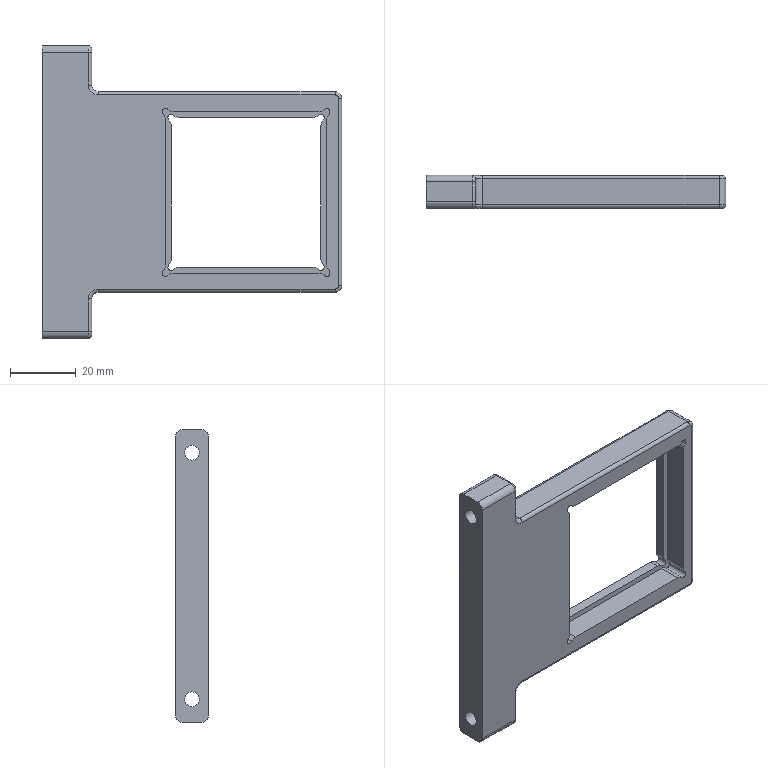CAM job | NX | 3+2 milling | part box 91 x 10 x 89 mm | stock box 96 x 12 x 90 mm
Tools:
number,name,description,diameter,corner_radius,flute_length,length,flutes
4,D4,平底铣刀-粗,4.0,0.0,25.0,75.0,2
9,D10,平底铣刀-粗,10.0,0.0,35.0,75.0,2
17,D2-J,平底铣刀-精,2.0,0.0,50.0,75.0,2
11,D4-J,平底铣刀-精,4.0,0.0,50.0,75.0,2
10,D10-J,平底铣刀-精,10.0,0.0,35.0,75.0,2
19,D4R0.5,圆鼻刀-粗,4.0,0.5,50.0,75.0,2
1,D80R0.8飞刀,圆鼻刀-粗,80.0,0.8,50.0,75.0,2
1,D80R0.8飞刀-J,圆鼻刀-精,80.0,0.8,50.0,75.0,2
2,D6倒角刀,倒角刀,6.0,0.0,3.0,25.0,2
Operations:
program,operation,operation_type,tool,method,geometry_group,spindle_rpm,surface_speed,feed_per_tooth,feed_cut,feed_plunge,cut_length_mm,path_length_mm,cut_time_min,machine_time_min
B,FLOORWALL_FACEMILL_ROUGH_COPY,VolumeBased25DMillingOperation,D80R0.8飞刀,LAYER_ROUGH-DEPTHK-STEPG,W-B,2800.0,703.696,0.5357,3000.0,100.0,1471.688,1680.498,0.4906,0.5114
B,FLOORWALL_FACEMILL_FINISH_COPY,VolumeBased25DMillingOperation,D80R0.8飞刀-J,SIDEFINISH-DEPTHK-STEPG,W-B,4000.0,1005.28,0.125,1000.0,100.0,367.285,463.285,0.3673,0.3769
B,ZLEVEL_FINISH_ZIGZAG_WALL_COPY_COPY_1,ZLevelMilling,D4R0.5,ZLEVEL_WALL-DEPTHK-STEPG,W-B,8000.0,100.531,0.25,4000.0,100.0,1678.657,1818.13,0.4197,0.4336
B,ZLEVEL_FINISH_ZIGZAG_WALL_COPY_COPY_COPY,ZLevelMilling,D4R0.5,ZLEVEL_WALL-DEPTHK-STEPG,W-B,8000.0,100.531,0.25,4000.0,100.0,5427.837,5452.449,1.357,1.359
B,PLANAR_DEBURR_6X45L_COPY,SurfaceContour,D6倒角刀,WALL_CHAMFER-DEPTH0-STEPG,W-B,6500.0,122.519,0.1154,1500.0,100.0,276.36,490.76,0.1842,0.2057
A,TOP_FACE,FaceMilling,D80R0.8飞刀,SIDEFINISH-DEPTHK-STEPG,W-A,4000.0,1005.31,0.125,1000.0,100.0,611.5,647.5,0.6115,0.6151
A,CAVITY_ROUGH_MID_COPY,CavityMilling,D10,LAYER_ROUGH-DEPTHK-STEPG,W-A,8000.0,251.327,0.1875,3000.0,100.0,9008.343,9587.592,3.003,3.092
A,CAVITY_ROUGH_MID_COPY_1,CavityMilling,D10,LAYER_ROUGH-DEPTHK-STEPG,W-A,8000.0,251.32,0.25,4000.0,100.0,23391.132,23910.636,5.848,5.926
A,CORNER_CLEAN_D4,ZLevelMilling,D4,METHOD,W-A,6000.0,75.0,0.25,2500.0,80.0,1067.761,1263.301,0.4275,0.4471
A,CORNER_CLEAN_D4_2,ZLevelMilling,D4,METHOD,W-A,6000.0,75.0,0.25,2500.0,80.0,438.591,621.874,0.1759,0.1942
A,PROFILE_SIDE,ZLevelMilling,D4-J,METHOD,W-A,9000.0,84.823,0.1389,2500.0,80.0,688.797,860.746,0.2757,0.2929
A,ZLEVEL_FINISH_ZIGZAG_WALL_COPY,ZLevelMilling,D4R0.5,ZLEVEL_WALL-DEPTHK-STEPG,W-A,8000.0,100.531,0.25,4000.0,100.0,1678.551,1811.625,0.4196,0.4329
A,ZLEVEL_FINISH_ZIGZAG_WALL_COPY_COPY,ZLevelMilling,D4R0.5,ZLEVEL_WALL-DEPTHK-STEPG,W-A,8000.0,100.531,0.25,4000.0,100.0,5427.851,5449.263,1.357,1.359
A,SELECTED_BODY_ONLY,SurfaceContour,D6倒角刀,METHOD,W-A,8000.0,150.796,0.1875,3000.0,100.0,291.381,454.275,0.0971,0.1134
A,FRAME_FINISH_1,VolumeBased25DMillingOperation,D4-J,METHOD,W-A,6000.0,113.0,0.0833,1000.0,100.0,171.423,230.423,0.1714,0.1773
A,BOTTOM_SIDE_FINISH_3,VolumeBased25DMillingOperation,D4-J,METHOD,W-A,6000.0,113.0,0.2083,1200.0,100.0,185.277,238.277,0.1544,0.1597
A,CORNER_CLEAN_D2,ZLevelMilling,D2-J,METHOD,W-A,9000.0,56.549,0.0667,1200.0,80.0,1602.181,1902.467,1.338,1.368
A,CORNER_CLEAN_D2_2,ZLevelMilling,D2-J,METHOD,W-A,9000.0,56.549,0.0667,1200.0,80.0,688.617,1018.423,0.5764,0.6094
A,PROFILE_SEMIFINISH_2,VolumeBased25DMillingOperation,D10-J,METHOD,W-A,8000.0,251.327,0.0625,1000.0,100.0,389.507,448.707,0.3895,0.3954